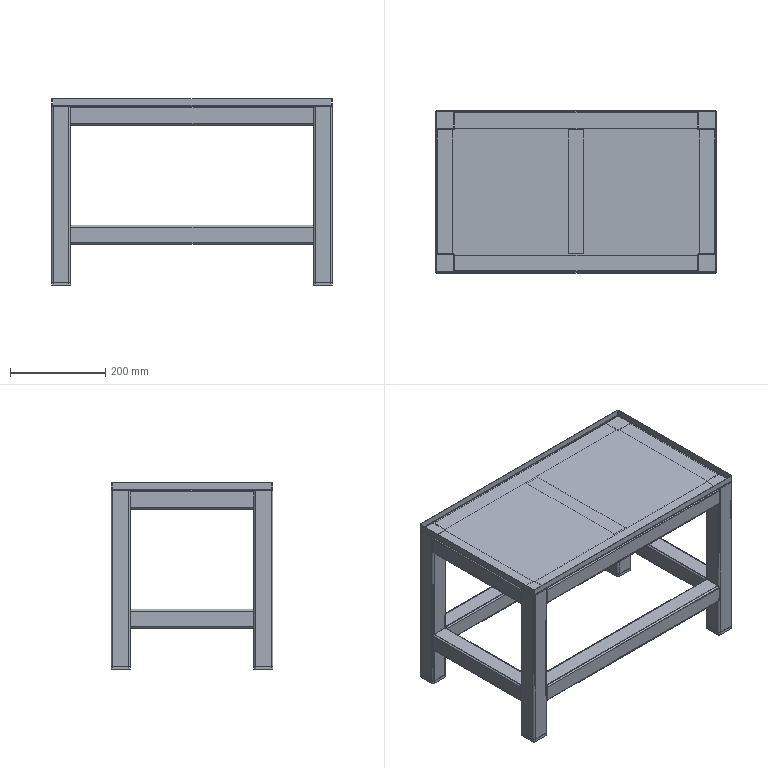Part | NX | features BREP 18 | 18 solids | 320 faces | box 590 x 340 x 391 mm | volume 1789604 mm3 | plane 176 | cylinder 136 | spline 8 | commonest cylinder face diameters 4 x56 8 x52 7 x16 6.8 x8 1 x4